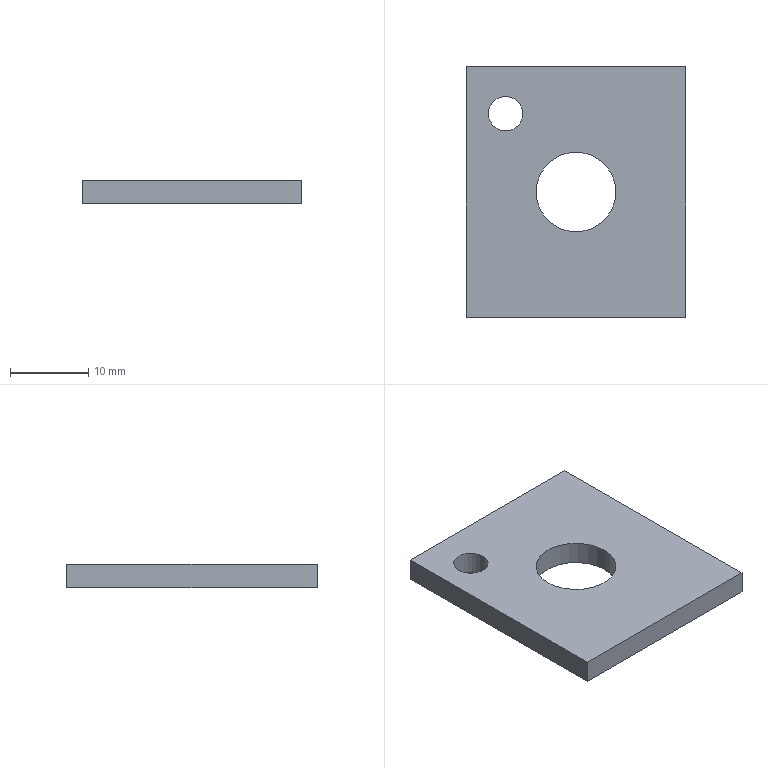Part | SolidWorks | features Extrusion 1, ICE 1 | 1 solid | 10 faces | box 28 x 32 x 3 mm | volume 2397 mm3 | plane 6 | cylinder 4 | commonest cylinder face diameters 4.4 x2 10.2 x2
STEP:
#1=CARTESIAN_POINT('',(-5.1,0.,-1.5));
#2=VERTEX_POINT('',#1);
#3=CARTESIAN_POINT('',(5.1,0.,-1.5));
#4=VERTEX_POINT('',#3);
#5=CARTESIAN_POINT('',(0.,0.,-1.5));
#6=DIRECTION('',(0.,0.,1.));
#7=DIRECTION('',(1.,0.,0.));
#8=AXIS2_PLACEMENT_3D('',#5,#6,#7);
#9=CIRCLE('',#8,5.1);
#10=EDGE_CURVE('',#2,#4,#9,.T.);
#11=ORIENTED_EDGE('',*,*,#10,.F.);
#12=CARTESIAN_POINT('',(-5.1,0.,1.5));
#13=VERTEX_POINT('',#12);
#14=CARTESIAN_POINT('',(-5.1,0.,-11.5));
#15=DIRECTION('',(0.,0.,1.));
#16=VECTOR('',#15,1000.);
#17=LINE('',#14,#16);
#18=EDGE_CURVE('',#2,#13,#17,.T.);
#19=ORIENTED_EDGE('',*,*,#18,.T.);
#20=CARTESIAN_POINT('',(5.1,0.,1.5));
#21=VERTEX_POINT('',#20);
#22=CARTESIAN_POINT('',(0.,0.,1.5));
#23=DIRECTION('',(0.,0.,1.));
#24=DIRECTION('',(1.,0.,0.));
#25=AXIS2_PLACEMENT_3D('',#22,#23,#24);
#26=CIRCLE('',#25,5.1);
#27=EDGE_CURVE('',#13,#21,#26,.T.);
#28=ORIENTED_EDGE('',*,*,#27,.T.);
#29=CARTESIAN_POINT('',(5.1,0.,-11.5));
#30=DIRECTION('',(0.,0.,1.));
#31=VECTOR('',#30,1000.);
#32=LINE('',#29,#31);
#33=EDGE_CURVE('',#4,#21,#32,.T.);
#34=ORIENTED_EDGE('',*,*,#33,.F.);
#35=EDGE_LOOP('',(#11,#19,#28,#34));
#36=FACE_OUTER_BOUND('',#35,.T.);
#37=CARTESIAN_POINT('',(0.,0.,-11.5));
#38=DIRECTION('',(0.,0.,1.));
#39=DIRECTION('',(1.,0.,0.));
#40=AXIS2_PLACEMENT_3D('',#37,#38,#39);
#41=CYLINDRICAL_SURFACE('',#40,5.1);
#42=ADVANCED_FACE('',(#36),#41,.F.);
#43=CARTESIAN_POINT('',(-11.2,10.,-1.5));
#44=VERTEX_POINT('',#43);
#45=CARTESIAN_POINT('',(-6.8,10.,-1.5));
#46=VERTEX_POINT('',#45);
#47=CARTESIAN_POINT('',(-9.,10.,-1.5));
#48=DIRECTION('',(0.,0.,1.));
#49=DIRECTION('',(1.,0.,0.));
#50=AXIS2_PLACEMENT_3D('',#47,#48,#49);
#51=CIRCLE('',#50,2.2);
#52=EDGE_CURVE('',#44,#46,#51,.T.);
#53=ORIENTED_EDGE('',*,*,#52,.F.);
#54=CARTESIAN_POINT('',(-11.2,10.,1.5));
#55=VERTEX_POINT('',#54);
#56=CARTESIAN_POINT('',(-11.2,10.,-11.5));
#57=DIRECTION('',(0.,0.,1.));
#58=VECTOR('',#57,1000.);
#59=LINE('',#56,#58);
#60=EDGE_CURVE('',#44,#55,#59,.T.);
#61=ORIENTED_EDGE('',*,*,#60,.T.);
#62=CARTESIAN_POINT('',(-6.8,10.,1.5));
#63=VERTEX_POINT('',#62);
#64=CARTESIAN_POINT('',(-9.,10.,1.5));
#65=DIRECTION('',(0.,0.,1.));
#66=DIRECTION('',(1.,0.,0.));
#67=AXIS2_PLACEMENT_3D('',#64,#65,#66);
#68=CIRCLE('',#67,2.2);
#69=EDGE_CURVE('',#55,#63,#68,.T.);
#70=ORIENTED_EDGE('',*,*,#69,.T.);
#71=CARTESIAN_POINT('',(-6.8,10.,-11.5));
#72=DIRECTION('',(0.,0.,1.));
#73=VECTOR('',#72,1000.);
#74=LINE('',#71,#73);
#75=EDGE_CURVE('',#46,#63,#74,.T.);
#76=ORIENTED_EDGE('',*,*,#75,.F.);
#77=EDGE_LOOP('',(#53,#61,#70,#76));
#78=FACE_OUTER_BOUND('',#77,.T.);
#79=CARTESIAN_POINT('',(-9.,10.,-11.5));
#80=DIRECTION('',(0.,0.,1.));
#81=DIRECTION('',(1.,0.,0.));
#82=AXIS2_PLACEMENT_3D('',#79,#80,#81);
#83=CYLINDRICAL_SURFACE('',#82,2.2);
#84=ADVANCED_FACE('',(#78),#83,.F.);
#85=CARTESIAN_POINT('',(-14.,16.,1.5));
#86=VERTEX_POINT('',#85);
#87=CARTESIAN_POINT('',(-14.,-16.,1.5));
#88=VERTEX_POINT('',#87);
#89=CARTESIAN_POINT('',(-14.,16.,1.5));
#90=DIRECTION('',(0.,-1.,0.));
#91=VECTOR('',#90,1000.);
#92=LINE('',#89,#91);
#93=EDGE_CURVE('',#86,#88,#92,.T.);
#94=ORIENTED_EDGE('',*,*,#93,.F.);
#95=CARTESIAN_POINT('',(-14.,16.,-1.5));
#96=VERTEX_POINT('',#95);
#97=CARTESIAN_POINT('',(-14.,16.,-1.5));
#98=DIRECTION('',(0.,0.,1.));
#99=VECTOR('',#98,1000.);
#100=LINE('',#97,#99);
#101=EDGE_CURVE('',#96,#86,#100,.T.);
#102=ORIENTED_EDGE('',*,*,#101,.F.);
#103=CARTESIAN_POINT('',(-14.,-16.,-1.5));
#104=VERTEX_POINT('',#103);
#105=CARTESIAN_POINT('',(-14.,16.,-1.5));
#106=DIRECTION('',(0.,-1.,0.));
#107=VECTOR('',#106,1000.);
#108=LINE('',#105,#107);
#109=EDGE_CURVE('',#96,#104,#108,.T.);
#110=ORIENTED_EDGE('',*,*,#109,.T.);
#111=CARTESIAN_POINT('',(-14.,-16.,-1.5));
#112=DIRECTION('',(0.,0.,1.));
#113=VECTOR('',#112,1000.);
#114=LINE('',#111,#113);
#115=EDGE_CURVE('',#104,#88,#114,.T.);
#116=ORIENTED_EDGE('',*,*,#115,.T.);
#117=EDGE_LOOP('',(#94,#102,#110,#116));
#118=FACE_OUTER_BOUND('',#117,.T.);
#119=CARTESIAN_POINT('',(-14.,16.,-1.5));
#120=DIRECTION('',(-1.,0.,0.));
#121=DIRECTION('',(0.,0.,1.));
#122=AXIS2_PLACEMENT_3D('',#119,#120,#121);
#123=PLANE('',#122);
#124=ADVANCED_FACE('',(#118),#123,.T.);
#125=CARTESIAN_POINT('',(14.,16.,1.5));
#126=VERTEX_POINT('',#125);
#127=CARTESIAN_POINT('',(14.,16.,1.5));
#128=DIRECTION('',(-1.,0.,0.));
#129=VECTOR('',#128,1000.);
#130=LINE('',#127,#129);
#131=EDGE_CURVE('',#126,#86,#130,.T.);
#132=ORIENTED_EDGE('',*,*,#131,.F.);
#133=CARTESIAN_POINT('',(14.,16.,-1.5));
#134=VERTEX_POINT('',#133);
#135=CARTESIAN_POINT('',(14.,16.,-1.5));
#136=DIRECTION('',(0.,0.,1.));
#137=VECTOR('',#136,1000.);
#138=LINE('',#135,#137);
#139=EDGE_CURVE('',#134,#126,#138,.T.);
#140=ORIENTED_EDGE('',*,*,#139,.F.);
#141=CARTESIAN_POINT('',(14.,16.,-1.5));
#142=DIRECTION('',(-1.,0.,0.));
#143=VECTOR('',#142,1000.);
#144=LINE('',#141,#143);
#145=EDGE_CURVE('',#134,#96,#144,.T.);
#146=ORIENTED_EDGE('',*,*,#145,.T.);
#147=ORIENTED_EDGE('',*,*,#101,.T.);
#148=EDGE_LOOP('',(#132,#140,#146,#147));
#149=FACE_OUTER_BOUND('',#148,.T.);
#150=CARTESIAN_POINT('',(14.,16.,-1.5));
#151=DIRECTION('',(0.,1.,0.));
#152=DIRECTION('',(0.,0.,1.));
#153=AXIS2_PLACEMENT_3D('',#150,#151,#152);
#154=PLANE('',#153);
#155=ADVANCED_FACE('',(#149),#154,.T.);
#156=CARTESIAN_POINT('',(14.,-16.,1.5));
#157=VERTEX_POINT('',#156);
#158=CARTESIAN_POINT('',(14.,-16.,1.5));
#159=DIRECTION('',(0.,1.,0.));
#160=VECTOR('',#159,1000.);
#161=LINE('',#158,#160);
#162=EDGE_CURVE('',#157,#126,#161,.T.);
#163=ORIENTED_EDGE('',*,*,#162,.F.);
#164=CARTESIAN_POINT('',(14.,-16.,-1.5));
#165=VERTEX_POINT('',#164);
#166=CARTESIAN_POINT('',(14.,-16.,-1.5));
#167=DIRECTION('',(0.,0.,1.));
#168=VECTOR('',#167,1000.);
#169=LINE('',#166,#168);
#170=EDGE_CURVE('',#165,#157,#169,.T.);
#171=ORIENTED_EDGE('',*,*,#170,.F.);
#172=CARTESIAN_POINT('',(14.,-16.,-1.5));
#173=DIRECTION('',(0.,1.,0.));
#174=VECTOR('',#173,1000.);
#175=LINE('',#172,#174);
#176=EDGE_CURVE('',#165,#134,#175,.T.);
#177=ORIENTED_EDGE('',*,*,#176,.T.);
#178=ORIENTED_EDGE('',*,*,#139,.T.);
#179=EDGE_LOOP('',(#163,#171,#177,#178));
#180=FACE_OUTER_BOUND('',#179,.T.);
#181=CARTESIAN_POINT('',(14.,-16.,-1.5));
#182=DIRECTION('',(1.,0.,0.));
#183=DIRECTION('',(0.,0.,-1.));
#184=AXIS2_PLACEMENT_3D('',#181,#182,#183);
#185=PLANE('',#184);
#186=ADVANCED_FACE('',(#180),#185,.T.);
#187=CARTESIAN_POINT('',(-14.,-16.,1.5));
#188=DIRECTION('',(1.,0.,0.));
#189=VECTOR('',#188,1000.);
#190=LINE('',#187,#189);
#191=EDGE_CURVE('',#88,#157,#190,.T.);
#192=ORIENTED_EDGE('',*,*,#191,.F.);
#193=ORIENTED_EDGE('',*,*,#115,.F.);
#194=CARTESIAN_POINT('',(-14.,-16.,-1.5));
#195=DIRECTION('',(1.,0.,0.));
#196=VECTOR('',#195,1000.);
#197=LINE('',#194,#196);
#198=EDGE_CURVE('',#104,#165,#197,.T.);
#199=ORIENTED_EDGE('',*,*,#198,.T.);
#200=ORIENTED_EDGE('',*,*,#170,.T.);
#201=EDGE_LOOP('',(#192,#193,#199,#200));
#202=FACE_OUTER_BOUND('',#201,.T.);
#203=CARTESIAN_POINT('',(-14.,-16.,-1.5));
#204=DIRECTION('',(0.,-1.,0.));
#205=DIRECTION('',(0.,0.,-1.));
#206=AXIS2_PLACEMENT_3D('',#203,#204,#205);
#207=PLANE('',#206);
#208=ADVANCED_FACE('',(#202),#207,.T.);
#209=CARTESIAN_POINT('',(0.,0.,-1.5));
#210=DIRECTION('',(0.,0.,1.));
#211=DIRECTION('',(1.,0.,0.));
#212=AXIS2_PLACEMENT_3D('',#209,#210,#211);
#213=CIRCLE('',#212,5.1);
#214=EDGE_CURVE('',#4,#2,#213,.T.);
#215=ORIENTED_EDGE('',*,*,#214,.T.);
#216=ORIENTED_EDGE('',*,*,#10,.T.);
#217=EDGE_LOOP('',(#215,#216));
#218=FACE_BOUND('',#217,.T.);
#219=CARTESIAN_POINT('',(-9.,10.,-1.5));
#220=DIRECTION('',(0.,0.,1.));
#221=DIRECTION('',(1.,0.,0.));
#222=AXIS2_PLACEMENT_3D('',#219,#220,#221);
#223=CIRCLE('',#222,2.2);
#224=EDGE_CURVE('',#46,#44,#223,.T.);
#225=ORIENTED_EDGE('',*,*,#224,.T.);
#226=ORIENTED_EDGE('',*,*,#52,.T.);
#227=EDGE_LOOP('',(#225,#226));
#228=FACE_BOUND('',#227,.T.);
#229=ORIENTED_EDGE('',*,*,#109,.F.);
#230=ORIENTED_EDGE('',*,*,#145,.F.);
#231=ORIENTED_EDGE('',*,*,#176,.F.);
#232=ORIENTED_EDGE('',*,*,#198,.F.);
#233=EDGE_LOOP('',(#229,#230,#231,#232));
#234=FACE_OUTER_BOUND('',#233,.T.);
#235=CARTESIAN_POINT('',(0.,0.,-1.5));
#236=DIRECTION('',(0.,0.,1.));
#237=DIRECTION('',(1.,0.,0.));
#238=AXIS2_PLACEMENT_3D('',#235,#236,#237);
#239=PLANE('',#238);
#240=ADVANCED_FACE('',(#218,#228,#234),#239,.F.);
#241=CARTESIAN_POINT('',(0.,0.,1.5));
#242=DIRECTION('',(0.,0.,1.));
#243=DIRECTION('',(1.,0.,0.));
#244=AXIS2_PLACEMENT_3D('',#241,#242,#243);
#245=CIRCLE('',#244,5.1);
#246=EDGE_CURVE('',#21,#13,#245,.T.);
#247=ORIENTED_EDGE('',*,*,#246,.F.);
#248=ORIENTED_EDGE('',*,*,#27,.F.);
#249=EDGE_LOOP('',(#247,#248));
#250=FACE_BOUND('',#249,.T.);
#251=CARTESIAN_POINT('',(-9.,10.,1.5));
#252=DIRECTION('',(0.,0.,1.));
#253=DIRECTION('',(1.,0.,0.));
#254=AXIS2_PLACEMENT_3D('',#251,#252,#253);
#255=CIRCLE('',#254,2.2);
#256=EDGE_CURVE('',#63,#55,#255,.T.);
#257=ORIENTED_EDGE('',*,*,#256,.F.);
#258=ORIENTED_EDGE('',*,*,#69,.F.);
#259=EDGE_LOOP('',(#257,#258));
#260=FACE_BOUND('',#259,.T.);
#261=ORIENTED_EDGE('',*,*,#93,.T.);
#262=ORIENTED_EDGE('',*,*,#191,.T.);
#263=ORIENTED_EDGE('',*,*,#162,.T.);
#264=ORIENTED_EDGE('',*,*,#131,.T.);
#265=EDGE_LOOP('',(#261,#262,#263,#264));
#266=FACE_OUTER_BOUND('',#265,.T.);
#267=CARTESIAN_POINT('',(0.,0.,1.5));
#268=DIRECTION('',(0.,0.,1.));
#269=DIRECTION('',(1.,0.,0.));
#270=AXIS2_PLACEMENT_3D('',#267,#268,#269);
#271=PLANE('',#270);
#272=ADVANCED_FACE('',(#250,#260,#266),#271,.T.);
#273=ORIENTED_EDGE('',*,*,#60,.F.);
#274=ORIENTED_EDGE('',*,*,#224,.F.);
#275=ORIENTED_EDGE('',*,*,#75,.T.);
#276=ORIENTED_EDGE('',*,*,#256,.T.);
#277=EDGE_LOOP('',(#273,#274,#275,#276));
#278=FACE_OUTER_BOUND('',#277,.T.);
#279=CARTESIAN_POINT('',(-9.,10.,-11.5));
#280=DIRECTION('',(0.,0.,1.));
#281=DIRECTION('',(1.,0.,0.));
#282=AXIS2_PLACEMENT_3D('',#279,#280,#281);
#283=CYLINDRICAL_SURFACE('',#282,2.2);
#284=ADVANCED_FACE('',(#278),#283,.F.);
#285=ORIENTED_EDGE('',*,*,#18,.F.);
#286=ORIENTED_EDGE('',*,*,#214,.F.);
#287=ORIENTED_EDGE('',*,*,#33,.T.);
#288=ORIENTED_EDGE('',*,*,#246,.T.);
#289=EDGE_LOOP('',(#285,#286,#287,#288));
#290=FACE_OUTER_BOUND('',#289,.T.);
#291=CARTESIAN_POINT('',(0.,0.,-11.5));
#292=DIRECTION('',(0.,0.,1.));
#293=DIRECTION('',(1.,0.,0.));
#294=AXIS2_PLACEMENT_3D('',#291,#292,#293);
#295=CYLINDRICAL_SURFACE('',#294,5.1);
#296=ADVANCED_FACE('',(#290),#295,.F.);
#297=CLOSED_SHELL('',(#42,#84,#124,#155,#186,#208,#240,#272,#284,#296));
#298=MANIFOLD_SOLID_BREP('',#297);
#299=CARTESIAN_POINT('',(0.,0.,0.));
#300=DIRECTION('',(0.,0.,1.));
#301=DIRECTION('',(1.,0.,0.));
#302=AXIS2_PLACEMENT_3D('',#299,#300,#301);
#303=(LENGTH_UNIT()NAMED_UNIT(*)SI_UNIT(.MILLI.,.METRE.));
#304=UNCERTAINTY_MEASURE_WITH_UNIT(LENGTH_MEASURE(0.00001),#303,'','');
#305=(NAMED_UNIT(*)PLANE_ANGLE_UNIT()SI_UNIT($,.RADIAN.));
#306=(NAMED_UNIT(*)SI_UNIT($,.STERADIAN.)SOLID_ANGLE_UNIT());
#307=(GEOMETRIC_REPRESENTATION_CONTEXT(3)GLOBAL_UNCERTAINTY_ASSIGNED_CONTEXT((#304))GLOBAL_UNIT_ASSIGNED_CONTEXT((#303,#305,#306))REPRESENTATION_CONTEXT('',''));
#308=ADVANCED_BREP_SHAPE_REPRESENTATION('',(#298,#302),#307);